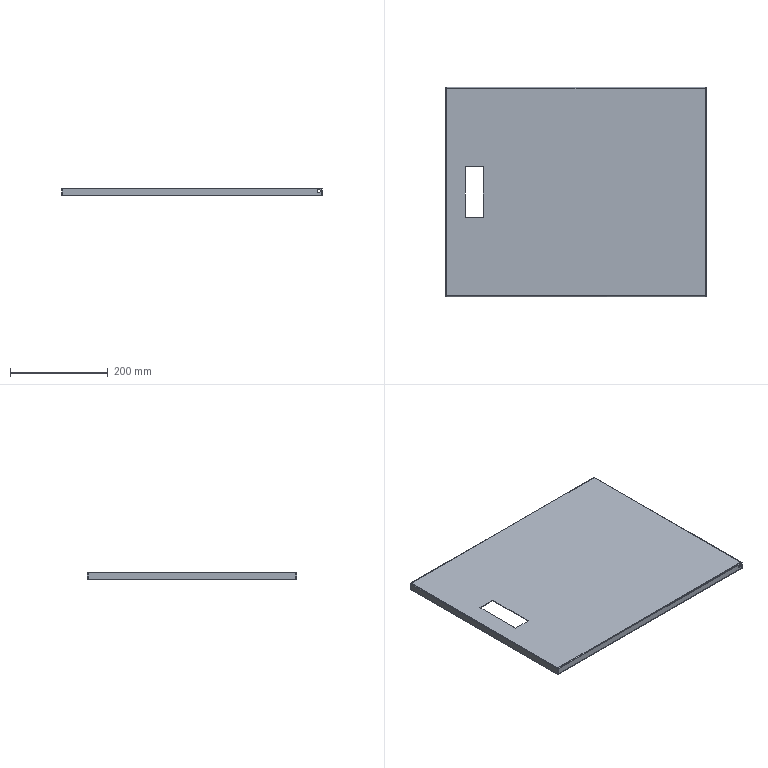Part | STEP file | 1 solid | 94 faces | box 533 x 428 x 16 mm | volume 320755 mm3 | plane 62 | cylinder 20 | spline 12 | commonest cylinder face diameters 1 x8 3.4 x8 6.5 x4